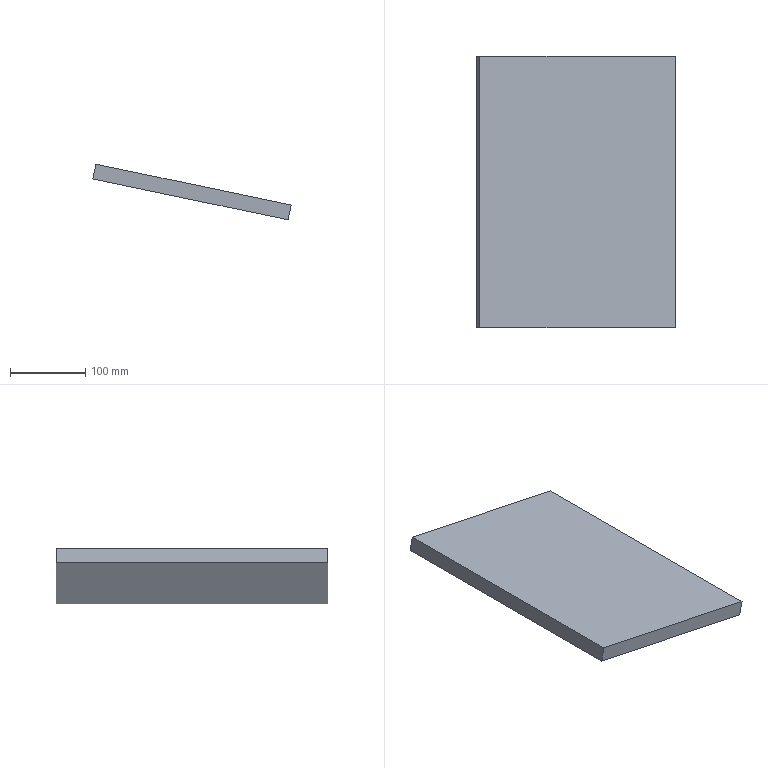Part | STEP file | 5_ESTAGIO_004-02 | 1 solid | 6 faces | box 263.449 x 360 x 74.068 mm | volume 1908000 mm3 | plane 6
STEP:
#1=CARTESIAN_POINT('',(0.,0.,0.));
#2=DIRECTION('',(0.,0.,1.));
#3=DIRECTION('',(1.,0.,0.));
#4=AXIS2_PLACEMENT_3D('',#1,#2,#3);
#5=CARTESIAN_POINT('',(-2604.907,-689.15,490.804));
#6=VERTEX_POINT('',#5);
#7=CARTESIAN_POINT('',(-2864.243,-689.15,545.3));
#8=VERTEX_POINT('',#7);
#9=CARTESIAN_POINT('',(-2604.907,-689.15,490.804));
#10=DIRECTION('',(-0.9786,0.,0.2056));
#11=VECTOR('',#10,1.);
#12=LINE('',#9,#11);
#13=CARTESIAN_POINT('',(-2600.794,-689.15,510.377));
#14=DIRECTION('',(0.,-1.,0.));
#15=DIRECTION('',(0.,0.,-1.));
#16=AXIS2_PLACEMENT_3D('',#13,#14,#15);
#17=PLANE('',#16);
#18=CARTESIAN_POINT('',(19.573,-4.113));
#19=DIRECTION('',(-0.2056,-0.9786));
#20=VECTOR('',#19,1.);
#21=LINE('',#18,#20);
#22=(GEOMETRIC_REPRESENTATION_CONTEXT(2)PARAMETRIC_REPRESENTATION_CONTEXT()REPRESENTATION_CONTEXT('',''));
#23=DEFINITIONAL_REPRESENTATION('',(#21),#22);
#24=PCURVE('',#17,#23);
#25=CARTESIAN_POINT('',(-11.386,0.,-54.184));
#26=DIRECTION('',(0.2056,0.,0.9786));
#27=DIRECTION('',(0.9786,0.,-0.2056));
#28=AXIS2_PLACEMENT_3D('',#25,#26,#27);
#29=PLANE('',#28);
#30=CARTESIAN_POINT('',(-2650.163,-689.15));
#31=DIRECTION('',(-1.,0.));
#32=VECTOR('',#31,1.);
#33=LINE('',#30,#32);
#34=(GEOMETRIC_REPRESENTATION_CONTEXT(2)PARAMETRIC_REPRESENTATION_CONTEXT()REPRESENTATION_CONTEXT('',''));
#35=DEFINITIONAL_REPRESENTATION('',(#33),#34);
#36=PCURVE('',#29,#35);
#37=SURFACE_CURVE('',#12,(#24,#36),.PCURVE_S1.);
#38=EDGE_CURVE('',#6,#8,#37,.T.);
#39=ORIENTED_EDGE('',*,*,#38,.T.);
#40=CARTESIAN_POINT('',(-2860.13,-689.15,564.872));
#41=VERTEX_POINT('',#40);
#42=CARTESIAN_POINT('',(-2860.13,-689.15,564.872));
#43=DIRECTION('',(-0.2056,0.,-0.9786));
#44=VECTOR('',#43,1.);
#45=LINE('',#42,#44);
#46=CARTESIAN_POINT('',(-54.495,-259.336));
#47=DIRECTION('',(0.9786,-0.2056));
#48=VECTOR('',#47,1.);
#49=LINE('',#46,#48);
#50=(GEOMETRIC_REPRESENTATION_CONTEXT(2)PARAMETRIC_REPRESENTATION_CONTEXT()REPRESENTATION_CONTEXT('',''));
#51=DEFINITIONAL_REPRESENTATION('',(#49),#50);
#52=PCURVE('',#17,#51);
#53=CARTESIAN_POINT('',(-2860.13,-1049.15,564.872));
#54=DIRECTION('',(-0.9786,0.,0.2056));
#55=DIRECTION('',(0.2056,0.,0.9786));
#56=AXIS2_PLACEMENT_3D('',#53,#54,#55);
#57=PLANE('',#56);
#58=CARTESIAN_POINT('',(0.,360.));
#59=DIRECTION('',(-1.,0.));
#60=VECTOR('',#59,1.);
#61=LINE('',#58,#60);
#62=(GEOMETRIC_REPRESENTATION_CONTEXT(2)PARAMETRIC_REPRESENTATION_CONTEXT()REPRESENTATION_CONTEXT('',''));
#63=DEFINITIONAL_REPRESENTATION('',(#61),#62);
#64=PCURVE('',#57,#63);
#65=SURFACE_CURVE('',#45,(#52,#64),.PCURVE_S1.);
#66=EDGE_CURVE('',#41,#8,#65,.T.);
#67=ORIENTED_EDGE('',*,*,#66,.F.);
#68=CARTESIAN_POINT('',(-2600.794,-689.15,510.377));
#69=VERTEX_POINT('',#68);
#70=CARTESIAN_POINT('',(-2600.794,-689.15,510.377));
#71=DIRECTION('',(-0.9786,0.,0.2056));
#72=VECTOR('',#71,1.);
#73=LINE('',#70,#72);
#74=CARTESIAN_POINT('',(0.,0.));
#75=DIRECTION('',(-0.2056,-0.9786));
#76=VECTOR('',#75,1.);
#77=LINE('',#74,#76);
#78=(GEOMETRIC_REPRESENTATION_CONTEXT(2)PARAMETRIC_REPRESENTATION_CONTEXT()REPRESENTATION_CONTEXT('',''));
#79=DEFINITIONAL_REPRESENTATION('',(#77),#78);
#80=PCURVE('',#17,#79);
#81=CARTESIAN_POINT('',(-7.273,0.,-34.611));
#82=DIRECTION('',(0.2056,0.,0.9786));
#83=DIRECTION('',(0.9786,0.,-0.2056));
#84=AXIS2_PLACEMENT_3D('',#81,#82,#83);
#85=PLANE('',#84);
#86=CARTESIAN_POINT('',(-2650.163,-689.15));
#87=DIRECTION('',(-1.,0.));
#88=VECTOR('',#87,1.);
#89=LINE('',#86,#88);
#90=(GEOMETRIC_REPRESENTATION_CONTEXT(2)PARAMETRIC_REPRESENTATION_CONTEXT()REPRESENTATION_CONTEXT('',''));
#91=DEFINITIONAL_REPRESENTATION('',(#89),#90);
#92=PCURVE('',#85,#91);
#93=SURFACE_CURVE('',#73,(#80,#92),.PCURVE_S1.);
#94=EDGE_CURVE('',#69,#41,#93,.T.);
#95=ORIENTED_EDGE('',*,*,#94,.F.);
#96=CARTESIAN_POINT('',(-2600.794,-689.15,510.377));
#97=DIRECTION('',(-0.2056,0.,-0.9786));
#98=VECTOR('',#97,1.);
#99=LINE('',#96,#98);
#100=CARTESIAN_POINT('',(0.,-0.000000001));
#101=DIRECTION('',(0.9786,-0.2056));
#102=VECTOR('',#101,1.);
#103=LINE('',#100,#102);
#104=(GEOMETRIC_REPRESENTATION_CONTEXT(2)PARAMETRIC_REPRESENTATION_CONTEXT()REPRESENTATION_CONTEXT('',''));
#105=DEFINITIONAL_REPRESENTATION('',(#103),#104);
#106=PCURVE('',#17,#105);
#107=CARTESIAN_POINT('',(-2600.794,-689.15,510.377));
#108=DIRECTION('',(0.9786,0.,-0.2056));
#109=DIRECTION('',(-0.2056,0.,-0.9786));
#110=AXIS2_PLACEMENT_3D('',#107,#108,#109);
#111=PLANE('',#110);
#112=CARTESIAN_POINT('',(0.,0.));
#113=DIRECTION('',(1.,0.));
#114=VECTOR('',#113,1.);
#115=LINE('',#112,#114);
#116=(GEOMETRIC_REPRESENTATION_CONTEXT(2)PARAMETRIC_REPRESENTATION_CONTEXT()REPRESENTATION_CONTEXT('',''));
#117=DEFINITIONAL_REPRESENTATION('',(#115),#116);
#118=PCURVE('',#111,#117);
#119=SURFACE_CURVE('',#99,(#106,#118),.PCURVE_S1.);
#120=EDGE_CURVE('',#69,#6,#119,.T.);
#121=ORIENTED_EDGE('',*,*,#120,.T.);
#122=EDGE_LOOP('',(#39,#67,#95,#121));
#123=FACE_BOUND('',#122,.T.);
#124=ADVANCED_FACE('',(#123),#17,.F.);
#125=CARTESIAN_POINT('',(-2864.243,-1049.15,545.3));
#126=VERTEX_POINT('',#125);
#127=CARTESIAN_POINT('',(-2864.243,-1049.15,545.3));
#128=DIRECTION('',(0.,1.,0.));
#129=VECTOR('',#128,1.);
#130=LINE('',#127,#129);
#131=CARTESIAN_POINT('',(-20.,0.));
#132=DIRECTION('',(0.,1.));
#133=VECTOR('',#132,1.);
#134=LINE('',#131,#133);
#135=(GEOMETRIC_REPRESENTATION_CONTEXT(2)PARAMETRIC_REPRESENTATION_CONTEXT()REPRESENTATION_CONTEXT('',''));
#136=DEFINITIONAL_REPRESENTATION('',(#134),#135);
#137=PCURVE('',#57,#136);
#138=CARTESIAN_POINT('',(-2915.163,-1049.15));
#139=DIRECTION('',(0.,1.));
#140=VECTOR('',#139,1.);
#141=LINE('',#138,#140);
#142=(GEOMETRIC_REPRESENTATION_CONTEXT(2)PARAMETRIC_REPRESENTATION_CONTEXT()REPRESENTATION_CONTEXT('',''));
#143=DEFINITIONAL_REPRESENTATION('',(#141),#142);
#144=PCURVE('',#29,#143);
#145=SURFACE_CURVE('',#130,(#137,#144),.PCURVE_S1.);
#146=EDGE_CURVE('',#126,#8,#145,.T.);
#147=ORIENTED_EDGE('',*,*,#146,.F.);
#148=CARTESIAN_POINT('',(-2860.13,-1049.15,564.872));
#149=VERTEX_POINT('',#148);
#150=CARTESIAN_POINT('',(-2860.13,-1049.15,564.872));
#151=DIRECTION('',(-0.2056,0.,-0.9786));
#152=VECTOR('',#151,1.);
#153=LINE('',#150,#152);
#154=CARTESIAN_POINT('',(0.,0.));
#155=DIRECTION('',(-1.,0.));
#156=VECTOR('',#155,1.);
#157=LINE('',#154,#156);
#158=(GEOMETRIC_REPRESENTATION_CONTEXT(2)PARAMETRIC_REPRESENTATION_CONTEXT()REPRESENTATION_CONTEXT('',''));
#159=DEFINITIONAL_REPRESENTATION('',(#157),#158);
#160=PCURVE('',#57,#159);
#161=CARTESIAN_POINT('',(-2860.13,-1049.15,564.872));
#162=DIRECTION('',(0.,1.,0.));
#163=DIRECTION('',(0.,0.,1.));
#164=AXIS2_PLACEMENT_3D('',#161,#162,#163);
#165=PLANE('',#164);
#166=CARTESIAN_POINT('',(0.,-0.000000001));
#167=DIRECTION('',(-0.9786,-0.2056));
#168=VECTOR('',#167,1.);
#169=LINE('',#166,#168);
#170=(GEOMETRIC_REPRESENTATION_CONTEXT(2)PARAMETRIC_REPRESENTATION_CONTEXT()REPRESENTATION_CONTEXT('',''));
#171=DEFINITIONAL_REPRESENTATION('',(#169),#170);
#172=PCURVE('',#165,#171);
#173=SURFACE_CURVE('',#153,(#160,#172),.PCURVE_S1.);
#174=EDGE_CURVE('',#149,#126,#173,.T.);
#175=ORIENTED_EDGE('',*,*,#174,.F.);
#176=CARTESIAN_POINT('',(-2860.13,-1049.15,564.872));
#177=DIRECTION('',(0.,1.,0.));
#178=VECTOR('',#177,1.);
#179=LINE('',#176,#178);
#180=CARTESIAN_POINT('',(0.,0.));
#181=DIRECTION('',(0.,1.));
#182=VECTOR('',#181,1.);
#183=LINE('',#180,#182);
#184=(GEOMETRIC_REPRESENTATION_CONTEXT(2)PARAMETRIC_REPRESENTATION_CONTEXT()REPRESENTATION_CONTEXT('',''));
#185=DEFINITIONAL_REPRESENTATION('',(#183),#184);
#186=PCURVE('',#57,#185);
#187=CARTESIAN_POINT('',(-2915.163,-1049.15));
#188=DIRECTION('',(0.,1.));
#189=VECTOR('',#188,1.);
#190=LINE('',#187,#189);
#191=(GEOMETRIC_REPRESENTATION_CONTEXT(2)PARAMETRIC_REPRESENTATION_CONTEXT()REPRESENTATION_CONTEXT('',''));
#192=DEFINITIONAL_REPRESENTATION('',(#190),#191);
#193=PCURVE('',#85,#192);
#194=SURFACE_CURVE('',#179,(#186,#193),.PCURVE_S1.);
#195=EDGE_CURVE('',#149,#41,#194,.T.);
#196=ORIENTED_EDGE('',*,*,#195,.T.);
#197=ORIENTED_EDGE('',*,*,#66,.T.);
#198=EDGE_LOOP('',(#147,#175,#196,#197));
#199=FACE_BOUND('',#198,.T.);
#200=ADVANCED_FACE('',(#199),#57,.T.);
#201=CARTESIAN_POINT('',(-2604.907,-1049.15,490.804));
#202=VERTEX_POINT('',#201);
#203=CARTESIAN_POINT('',(-2864.243,-1049.15,545.3));
#204=DIRECTION('',(0.9786,0.,-0.2056));
#205=VECTOR('',#204,1.);
#206=LINE('',#203,#205);
#207=CARTESIAN_POINT('',(-19.573,-4.113));
#208=DIRECTION('',(-0.2056,0.9786));
#209=VECTOR('',#208,1.);
#210=LINE('',#207,#209);
#211=(GEOMETRIC_REPRESENTATION_CONTEXT(2)PARAMETRIC_REPRESENTATION_CONTEXT()REPRESENTATION_CONTEXT('',''));
#212=DEFINITIONAL_REPRESENTATION('',(#210),#211);
#213=PCURVE('',#165,#212);
#214=CARTESIAN_POINT('',(-2915.163,-1049.15));
#215=DIRECTION('',(1.,0.));
#216=VECTOR('',#215,1.);
#217=LINE('',#214,#216);
#218=(GEOMETRIC_REPRESENTATION_CONTEXT(2)PARAMETRIC_REPRESENTATION_CONTEXT()REPRESENTATION_CONTEXT('',''));
#219=DEFINITIONAL_REPRESENTATION('',(#217),#218);
#220=PCURVE('',#29,#219);
#221=SURFACE_CURVE('',#206,(#213,#220),.PCURVE_S1.);
#222=EDGE_CURVE('',#126,#202,#221,.T.);
#223=ORIENTED_EDGE('',*,*,#222,.T.);
#224=CARTESIAN_POINT('',(-2600.794,-1049.15,510.377));
#225=VERTEX_POINT('',#224);
#226=CARTESIAN_POINT('',(-2600.794,-1049.15,510.377));
#227=DIRECTION('',(-0.2056,0.,-0.9786));
#228=VECTOR('',#227,1.);
#229=LINE('',#226,#228);
#230=CARTESIAN_POINT('',(-54.495,259.336));
#231=DIRECTION('',(-0.9786,-0.2056));
#232=VECTOR('',#231,1.);
#233=LINE('',#230,#232);
#234=(GEOMETRIC_REPRESENTATION_CONTEXT(2)PARAMETRIC_REPRESENTATION_CONTEXT()REPRESENTATION_CONTEXT('',''));
#235=DEFINITIONAL_REPRESENTATION('',(#233),#234);
#236=PCURVE('',#165,#235);
#237=CARTESIAN_POINT('',(0.,-360.));
#238=DIRECTION('',(1.,0.));
#239=VECTOR('',#238,1.);
#240=LINE('',#237,#239);
#241=(GEOMETRIC_REPRESENTATION_CONTEXT(2)PARAMETRIC_REPRESENTATION_CONTEXT()REPRESENTATION_CONTEXT('',''));
#242=DEFINITIONAL_REPRESENTATION('',(#240),#241);
#243=PCURVE('',#111,#242);
#244=SURFACE_CURVE('',#229,(#236,#243),.PCURVE_S1.);
#245=EDGE_CURVE('',#225,#202,#244,.T.);
#246=ORIENTED_EDGE('',*,*,#245,.F.);
#247=CARTESIAN_POINT('',(-2860.13,-1049.15,564.872));
#248=DIRECTION('',(0.9786,0.,-0.2056));
#249=VECTOR('',#248,1.);
#250=LINE('',#247,#249);
#251=CARTESIAN_POINT('',(-0.000000001,-0.000000001));
#252=DIRECTION('',(-0.2056,0.9786));
#253=VECTOR('',#252,1.);
#254=LINE('',#251,#253);
#255=(GEOMETRIC_REPRESENTATION_CONTEXT(2)PARAMETRIC_REPRESENTATION_CONTEXT()REPRESENTATION_CONTEXT('',''));
#256=DEFINITIONAL_REPRESENTATION('',(#254),#255);
#257=PCURVE('',#165,#256);
#258=CARTESIAN_POINT('',(-2915.163,-1049.15));
#259=DIRECTION('',(1.,0.));
#260=VECTOR('',#259,1.);
#261=LINE('',#258,#260);
#262=(GEOMETRIC_REPRESENTATION_CONTEXT(2)PARAMETRIC_REPRESENTATION_CONTEXT()REPRESENTATION_CONTEXT('',''));
#263=DEFINITIONAL_REPRESENTATION('',(#261),#262);
#264=PCURVE('',#85,#263);
#265=SURFACE_CURVE('',#250,(#257,#264),.PCURVE_S1.);
#266=EDGE_CURVE('',#149,#225,#265,.T.);
#267=ORIENTED_EDGE('',*,*,#266,.F.);
#268=ORIENTED_EDGE('',*,*,#174,.T.);
#269=EDGE_LOOP('',(#223,#246,#267,#268));
#270=FACE_BOUND('',#269,.T.);
#271=ADVANCED_FACE('',(#270),#165,.F.);
#272=CARTESIAN_POINT('',(-2604.907,-689.15,490.804));
#273=DIRECTION('',(0.,-1.,0.));
#274=VECTOR('',#273,1.);
#275=LINE('',#272,#274);
#276=CARTESIAN_POINT('',(20.,0.));
#277=DIRECTION('',(0.,-1.));
#278=VECTOR('',#277,1.);
#279=LINE('',#276,#278);
#280=(GEOMETRIC_REPRESENTATION_CONTEXT(2)PARAMETRIC_REPRESENTATION_CONTEXT()REPRESENTATION_CONTEXT('',''));
#281=DEFINITIONAL_REPRESENTATION('',(#279),#280);
#282=PCURVE('',#111,#281);
#283=CARTESIAN_POINT('',(-2650.163,-689.15));
#284=DIRECTION('',(0.,-1.));
#285=VECTOR('',#284,1.);
#286=LINE('',#283,#285);
#287=(GEOMETRIC_REPRESENTATION_CONTEXT(2)PARAMETRIC_REPRESENTATION_CONTEXT()REPRESENTATION_CONTEXT('',''));
#288=DEFINITIONAL_REPRESENTATION('',(#286),#287);
#289=PCURVE('',#29,#288);
#290=SURFACE_CURVE('',#275,(#282,#289),.PCURVE_S1.);
#291=EDGE_CURVE('',#6,#202,#290,.T.);
#292=ORIENTED_EDGE('',*,*,#291,.F.);
#293=ORIENTED_EDGE('',*,*,#120,.F.);
#294=CARTESIAN_POINT('',(-2600.794,-689.15,510.377));
#295=DIRECTION('',(0.,-1.,0.));
#296=VECTOR('',#295,1.);
#297=LINE('',#294,#296);
#298=CARTESIAN_POINT('',(0.,0.));
#299=DIRECTION('',(0.,-1.));
#300=VECTOR('',#299,1.);
#301=LINE('',#298,#300);
#302=(GEOMETRIC_REPRESENTATION_CONTEXT(2)PARAMETRIC_REPRESENTATION_CONTEXT()REPRESENTATION_CONTEXT('',''));
#303=DEFINITIONAL_REPRESENTATION('',(#301),#302);
#304=PCURVE('',#111,#303);
#305=CARTESIAN_POINT('',(-2650.163,-689.15));
#306=DIRECTION('',(0.,-1.));
#307=VECTOR('',#306,1.);
#308=LINE('',#305,#307);
#309=(GEOMETRIC_REPRESENTATION_CONTEXT(2)PARAMETRIC_REPRESENTATION_CONTEXT()REPRESENTATION_CONTEXT('',''));
#310=DEFINITIONAL_REPRESENTATION('',(#308),#309);
#311=PCURVE('',#85,#310);
#312=SURFACE_CURVE('',#297,(#304,#311),.PCURVE_S1.);
#313=EDGE_CURVE('',#69,#225,#312,.T.);
#314=ORIENTED_EDGE('',*,*,#313,.T.);
#315=ORIENTED_EDGE('',*,*,#245,.T.);
#316=EDGE_LOOP('',(#292,#293,#314,#315));
#317=FACE_BOUND('',#316,.T.);
#318=ADVANCED_FACE('',(#317),#111,.T.);
#319=ORIENTED_EDGE('',*,*,#94,.T.);
#320=ORIENTED_EDGE('',*,*,#195,.F.);
#321=ORIENTED_EDGE('',*,*,#266,.T.);
#322=ORIENTED_EDGE('',*,*,#313,.F.);
#323=EDGE_LOOP('',(#319,#320,#321,#322));
#324=FACE_BOUND('',#323,.T.);
#325=ADVANCED_FACE('',(#324),#85,.T.);
#326=ORIENTED_EDGE('',*,*,#291,.T.);
#327=ORIENTED_EDGE('',*,*,#222,.F.);
#328=ORIENTED_EDGE('',*,*,#146,.T.);
#329=ORIENTED_EDGE('',*,*,#38,.F.);
#330=EDGE_LOOP('',(#326,#327,#328,#329));
#331=FACE_BOUND('',#330,.T.);
#332=ADVANCED_FACE('',(#331),#29,.F.);
#333=CLOSED_SHELL('',(#124,#200,#271,#318,#325,#332));
#334=MANIFOLD_SOLID_BREP('',#333);
#335=(LENGTH_UNIT()NAMED_UNIT(*)SI_UNIT(.MILLI.,.METRE.));
#336=UNCERTAINTY_MEASURE_WITH_UNIT(LENGTH_MEASURE(0.0000001),#335,'','');
#337=(NAMED_UNIT(*)PLANE_ANGLE_UNIT()SI_UNIT($,.RADIAN.));
#338=(NAMED_UNIT(*)SI_UNIT($,.STERADIAN.)SOLID_ANGLE_UNIT());
#339=(GEOMETRIC_REPRESENTATION_CONTEXT(3)GLOBAL_UNCERTAINTY_ASSIGNED_CONTEXT((#336))GLOBAL_UNIT_ASSIGNED_CONTEXT((#335,#337,#338))REPRESENTATION_CONTEXT('',''));
#340=ADVANCED_BREP_SHAPE_REPRESENTATION('',(#4,#334),#339);